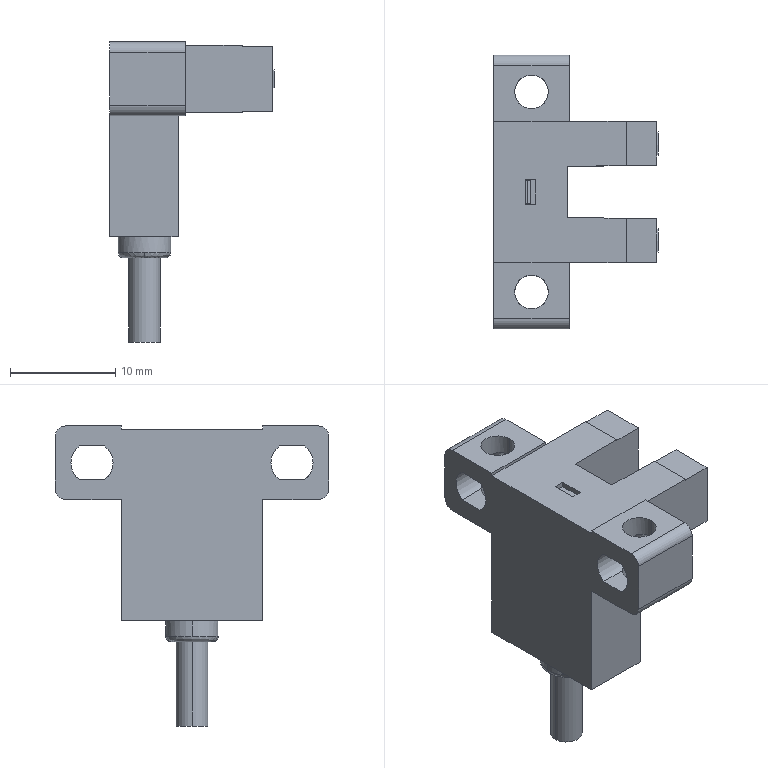Part | SolidWorks | features BaseBody 3, ICE 1 | 1 solid | 104 faces | box 15.65 x 26 x 28.5 mm | volume 2575 mm3 | plane 77 | cylinder 23 | spline 2 | cone 2 | commonest cylinder face diameters 3.2 x8 2 x4 4 x4 2.8 x2 3 x2 5 x2